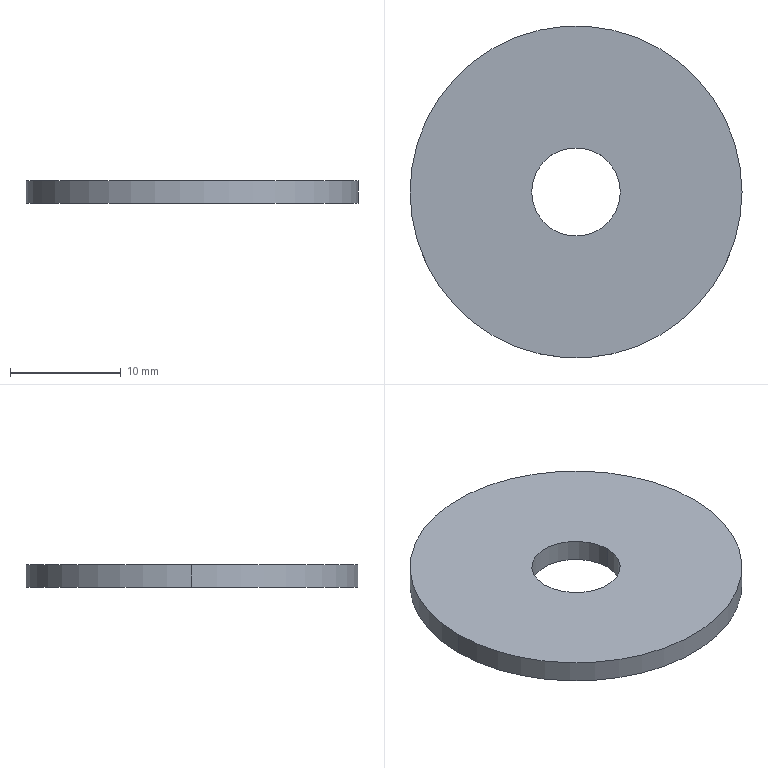Part | STEP file | BCC3 H16_6 | 1 solid | 6 faces | box 30 x 30 x 2 mm | volume 1313 mm3 | cylinder 4 | plane 2 | commonest cylinder face diameters 8 x2 30 x2
STEP:
#1=CARTESIAN_POINT('',(0.,0.,0.));
#2=DIRECTION('',(0.,0.,1.));
#3=DIRECTION('',(1.,0.,0.));
#4=AXIS2_PLACEMENT_3D('',#1,#2,#3);
#5=CARTESIAN_POINT('',(-4.,0.,2.));
#6=VERTEX_POINT('',#5);
#7=CARTESIAN_POINT('',(-4.,0.,0.));
#8=VERTEX_POINT('',#7);
#9=CARTESIAN_POINT('',(-4.,0.,2.));
#10=DIRECTION('',(0.,0.,-1.));
#11=VECTOR('',#10,1.);
#12=LINE('',#9,#11);
#13=CARTESIAN_POINT('',(0.,0.,2.));
#14=DIRECTION('',(0.,0.,-1.));
#15=DIRECTION('',(-1.,0.,0.));
#16=AXIS2_PLACEMENT_3D('',#13,#14,#15);
#17=CYLINDRICAL_SURFACE('',#16,4.);
#18=CARTESIAN_POINT('',(6.283,0.));
#19=DIRECTION('',(0.,1.));
#20=VECTOR('',#19,1.);
#21=LINE('',#18,#20);
#22=(GEOMETRIC_REPRESENTATION_CONTEXT(2)PARAMETRIC_REPRESENTATION_CONTEXT()REPRESENTATION_CONTEXT('',''));
#23=DEFINITIONAL_REPRESENTATION('',(#21),#22);
#24=PCURVE('',#17,#23);
#25=CARTESIAN_POINT('',(0.,0.,2.));
#26=DIRECTION('',(0.,0.,-1.));
#27=DIRECTION('',(-1.,0.,0.));
#28=AXIS2_PLACEMENT_3D('',#25,#26,#27);
#29=CYLINDRICAL_SURFACE('',#28,4.);
#30=CARTESIAN_POINT('',(0.,0.));
#31=DIRECTION('',(0.,1.));
#32=VECTOR('',#31,1.);
#33=LINE('',#30,#32);
#34=(GEOMETRIC_REPRESENTATION_CONTEXT(2)PARAMETRIC_REPRESENTATION_CONTEXT()REPRESENTATION_CONTEXT('',''));
#35=DEFINITIONAL_REPRESENTATION('',(#33),#34);
#36=PCURVE('',#29,#35);
#37=SURFACE_CURVE('',#12,(#24,#36),.PCURVE_S1.);
#38=EDGE_CURVE('',#6,#8,#37,.T.);
#39=ORIENTED_EDGE('',*,*,#38,.T.);
#40=CARTESIAN_POINT('',(4.,0.,0.));
#41=VERTEX_POINT('',#40);
#42=CARTESIAN_POINT('',(0.,0.,0.));
#43=DIRECTION('',(0.,0.,1.));
#44=DIRECTION('',(1.,0.,0.));
#45=AXIS2_PLACEMENT_3D('',#42,#43,#44);
#46=CIRCLE('',#45,4.);
#47=CARTESIAN_POINT('',(9.425,2.));
#48=DIRECTION('',(-1.,0.));
#49=VECTOR('',#48,1.);
#50=LINE('',#47,#49);
#51=(GEOMETRIC_REPRESENTATION_CONTEXT(2)PARAMETRIC_REPRESENTATION_CONTEXT()REPRESENTATION_CONTEXT('',''));
#52=DEFINITIONAL_REPRESENTATION('',(#50),#51);
#53=PCURVE('',#17,#52);
#54=CARTESIAN_POINT('',(0.,0.,0.));
#55=DIRECTION('',(0.,0.,1.));
#56=DIRECTION('',(1.,0.,0.));
#57=AXIS2_PLACEMENT_3D('',#54,#55,#56);
#58=PLANE('',#57);
#59=CARTESIAN_POINT('',(0.,0.));
#60=DIRECTION('',(1.,0.));
#61=AXIS2_PLACEMENT_2D('',#59,#60);
#62=CIRCLE('',#61,4.);
#63=(GEOMETRIC_REPRESENTATION_CONTEXT(2)PARAMETRIC_REPRESENTATION_CONTEXT()REPRESENTATION_CONTEXT('',''));
#64=DEFINITIONAL_REPRESENTATION('',(#62),#63);
#65=PCURVE('',#58,#64);
#66=SURFACE_CURVE('',#46,(#53,#65),.PCURVE_S1.);
#67=EDGE_CURVE('',#8,#41,#66,.T.);
#68=ORIENTED_EDGE('',*,*,#67,.T.);
#69=CARTESIAN_POINT('',(4.,0.,2.));
#70=VERTEX_POINT('',#69);
#71=CARTESIAN_POINT('',(4.,0.,2.));
#72=DIRECTION('',(0.,0.,-1.));
#73=VECTOR('',#72,1.);
#74=LINE('',#71,#73);
#75=CARTESIAN_POINT('',(3.142,0.));
#76=DIRECTION('',(0.,1.));
#77=VECTOR('',#76,1.);
#78=LINE('',#75,#77);
#79=(GEOMETRIC_REPRESENTATION_CONTEXT(2)PARAMETRIC_REPRESENTATION_CONTEXT()REPRESENTATION_CONTEXT('',''));
#80=DEFINITIONAL_REPRESENTATION('',(#78),#79);
#81=PCURVE('',#17,#80);
#82=CARTESIAN_POINT('',(3.142,0.));
#83=DIRECTION('',(0.,1.));
#84=VECTOR('',#83,1.);
#85=LINE('',#82,#84);
#86=(GEOMETRIC_REPRESENTATION_CONTEXT(2)PARAMETRIC_REPRESENTATION_CONTEXT()REPRESENTATION_CONTEXT('',''));
#87=DEFINITIONAL_REPRESENTATION('',(#85),#86);
#88=PCURVE('',#29,#87);
#89=SURFACE_CURVE('',#74,(#81,#88),.PCURVE_S1.);
#90=EDGE_CURVE('',#70,#41,#89,.T.);
#91=ORIENTED_EDGE('',*,*,#90,.F.);
#92=CARTESIAN_POINT('',(0.,0.,2.));
#93=DIRECTION('',(0.,0.,1.));
#94=DIRECTION('',(1.,0.,0.));
#95=AXIS2_PLACEMENT_3D('',#92,#93,#94);
#96=CIRCLE('',#95,4.);
#97=CARTESIAN_POINT('',(9.425,0.));
#98=DIRECTION('',(-1.,0.));
#99=VECTOR('',#98,1.);
#100=LINE('',#97,#99);
#101=(GEOMETRIC_REPRESENTATION_CONTEXT(2)PARAMETRIC_REPRESENTATION_CONTEXT()REPRESENTATION_CONTEXT('',''));
#102=DEFINITIONAL_REPRESENTATION('',(#100),#101);
#103=PCURVE('',#17,#102);
#104=CARTESIAN_POINT('',(0.,0.,2.));
#105=DIRECTION('',(0.,0.,1.));
#106=DIRECTION('',(1.,0.,0.));
#107=AXIS2_PLACEMENT_3D('',#104,#105,#106);
#108=PLANE('',#107);
#109=CARTESIAN_POINT('',(0.,0.));
#110=DIRECTION('',(1.,0.));
#111=AXIS2_PLACEMENT_2D('',#109,#110);
#112=CIRCLE('',#111,4.);
#113=(GEOMETRIC_REPRESENTATION_CONTEXT(2)PARAMETRIC_REPRESENTATION_CONTEXT()REPRESENTATION_CONTEXT('',''));
#114=DEFINITIONAL_REPRESENTATION('',(#112),#113);
#115=PCURVE('',#108,#114);
#116=SURFACE_CURVE('',#96,(#103,#115),.PCURVE_S1.);
#117=EDGE_CURVE('',#6,#70,#116,.T.);
#118=ORIENTED_EDGE('',*,*,#117,.F.);
#119=EDGE_LOOP('',(#39,#68,#91,#118));
#120=FACE_BOUND('',#119,.F.);
#121=ADVANCED_FACE('',(#120),#17,.F.);
#122=CARTESIAN_POINT('',(15.,0.,2.));
#123=VERTEX_POINT('',#122);
#124=CARTESIAN_POINT('',(-15.,0.,2.));
#125=VERTEX_POINT('',#124);
#126=CARTESIAN_POINT('',(0.,0.,2.));
#127=DIRECTION('',(0.,0.,1.));
#128=DIRECTION('',(1.,0.,0.));
#129=AXIS2_PLACEMENT_3D('',#126,#127,#128);
#130=CIRCLE('',#129,15.);
#131=CARTESIAN_POINT('',(0.,0.,2.));
#132=DIRECTION('',(0.,0.,-1.));
#133=DIRECTION('',(-1.,0.,0.));
#134=AXIS2_PLACEMENT_3D('',#131,#132,#133);
#135=CYLINDRICAL_SURFACE('',#134,15.);
#136=CARTESIAN_POINT('',(3.142,0.));
#137=DIRECTION('',(-1.,0.));
#138=VECTOR('',#137,1.);
#139=LINE('',#136,#138);
#140=(GEOMETRIC_REPRESENTATION_CONTEXT(2)PARAMETRIC_REPRESENTATION_CONTEXT()REPRESENTATION_CONTEXT('',''));
#141=DEFINITIONAL_REPRESENTATION('',(#139),#140);
#142=PCURVE('',#135,#141);
#143=CARTESIAN_POINT('',(0.,0.));
#144=DIRECTION('',(1.,0.));
#145=AXIS2_PLACEMENT_2D('',#143,#144);
#146=CIRCLE('',#145,15.);
#147=(GEOMETRIC_REPRESENTATION_CONTEXT(2)PARAMETRIC_REPRESENTATION_CONTEXT()REPRESENTATION_CONTEXT('',''));
#148=DEFINITIONAL_REPRESENTATION('',(#146),#147);
#149=PCURVE('',#108,#148);
#150=SURFACE_CURVE('',#130,(#142,#149),.PCURVE_S1.);
#151=EDGE_CURVE('',#123,#125,#150,.T.);
#152=ORIENTED_EDGE('',*,*,#151,.F.);
#153=CARTESIAN_POINT('',(15.,0.,0.));
#154=VERTEX_POINT('',#153);
#155=CARTESIAN_POINT('',(15.,0.,2.));
#156=DIRECTION('',(0.,0.,-1.));
#157=VECTOR('',#156,1.);
#158=LINE('',#155,#157);
#159=CARTESIAN_POINT('',(3.142,0.));
#160=DIRECTION('',(0.,1.));
#161=VECTOR('',#160,1.);
#162=LINE('',#159,#161);
#163=(GEOMETRIC_REPRESENTATION_CONTEXT(2)PARAMETRIC_REPRESENTATION_CONTEXT()REPRESENTATION_CONTEXT('',''));
#164=DEFINITIONAL_REPRESENTATION('',(#162),#163);
#165=PCURVE('',#135,#164);
#166=CARTESIAN_POINT('',(0.,0.,2.));
#167=DIRECTION('',(0.,0.,-1.));
#168=DIRECTION('',(-1.,0.,0.));
#169=AXIS2_PLACEMENT_3D('',#166,#167,#168);
#170=CYLINDRICAL_SURFACE('',#169,15.);
#171=CARTESIAN_POINT('',(3.142,0.));
#172=DIRECTION('',(0.,1.));
#173=VECTOR('',#172,1.);
#174=LINE('',#171,#173);
#175=(GEOMETRIC_REPRESENTATION_CONTEXT(2)PARAMETRIC_REPRESENTATION_CONTEXT()REPRESENTATION_CONTEXT('',''));
#176=DEFINITIONAL_REPRESENTATION('',(#174),#175);
#177=PCURVE('',#170,#176);
#178=SURFACE_CURVE('',#158,(#165,#177),.PCURVE_S1.);
#179=EDGE_CURVE('',#123,#154,#178,.T.);
#180=ORIENTED_EDGE('',*,*,#179,.T.);
#181=CARTESIAN_POINT('',(-15.,0.,0.));
#182=VERTEX_POINT('',#181);
#183=CARTESIAN_POINT('',(0.,0.,0.));
#184=DIRECTION('',(0.,0.,1.));
#185=DIRECTION('',(1.,0.,0.));
#186=AXIS2_PLACEMENT_3D('',#183,#184,#185);
#187=CIRCLE('',#186,15.);
#188=CARTESIAN_POINT('',(3.142,2.));
#189=DIRECTION('',(-1.,0.));
#190=VECTOR('',#189,1.);
#191=LINE('',#188,#190);
#192=(GEOMETRIC_REPRESENTATION_CONTEXT(2)PARAMETRIC_REPRESENTATION_CONTEXT()REPRESENTATION_CONTEXT('',''));
#193=DEFINITIONAL_REPRESENTATION('',(#191),#192);
#194=PCURVE('',#135,#193);
#195=CARTESIAN_POINT('',(0.,0.));
#196=DIRECTION('',(1.,0.));
#197=AXIS2_PLACEMENT_2D('',#195,#196);
#198=CIRCLE('',#197,15.);
#199=(GEOMETRIC_REPRESENTATION_CONTEXT(2)PARAMETRIC_REPRESENTATION_CONTEXT()REPRESENTATION_CONTEXT('',''));
#200=DEFINITIONAL_REPRESENTATION('',(#198),#199);
#201=PCURVE('',#58,#200);
#202=SURFACE_CURVE('',#187,(#194,#201),.PCURVE_S1.);
#203=EDGE_CURVE('',#154,#182,#202,.T.);
#204=ORIENTED_EDGE('',*,*,#203,.T.);
#205=CARTESIAN_POINT('',(-15.,0.,2.));
#206=DIRECTION('',(0.,0.,-1.));
#207=VECTOR('',#206,1.);
#208=LINE('',#205,#207);
#209=CARTESIAN_POINT('',(0.,0.));
#210=DIRECTION('',(0.,1.));
#211=VECTOR('',#210,1.);
#212=LINE('',#209,#211);
#213=(GEOMETRIC_REPRESENTATION_CONTEXT(2)PARAMETRIC_REPRESENTATION_CONTEXT()REPRESENTATION_CONTEXT('',''));
#214=DEFINITIONAL_REPRESENTATION('',(#212),#213);
#215=PCURVE('',#135,#214);
#216=CARTESIAN_POINT('',(6.283,0.));
#217=DIRECTION('',(0.,1.));
#218=VECTOR('',#217,1.);
#219=LINE('',#216,#218);
#220=(GEOMETRIC_REPRESENTATION_CONTEXT(2)PARAMETRIC_REPRESENTATION_CONTEXT()REPRESENTATION_CONTEXT('',''));
#221=DEFINITIONAL_REPRESENTATION('',(#219),#220);
#222=PCURVE('',#170,#221);
#223=SURFACE_CURVE('',#208,(#215,#222),.PCURVE_S1.);
#224=EDGE_CURVE('',#125,#182,#223,.T.);
#225=ORIENTED_EDGE('',*,*,#224,.F.);
#226=EDGE_LOOP('',(#152,#180,#204,#225));
#227=FACE_BOUND('',#226,.T.);
#228=ADVANCED_FACE('',(#227),#135,.T.);
#229=CARTESIAN_POINT('',(0.,0.,2.));
#230=DIRECTION('',(0.,0.,1.));
#231=DIRECTION('',(1.,0.,0.));
#232=AXIS2_PLACEMENT_3D('',#229,#230,#231);
#233=CIRCLE('',#232,15.);
#234=CARTESIAN_POINT('',(0.,0.));
#235=DIRECTION('',(1.,0.));
#236=AXIS2_PLACEMENT_2D('',#234,#235);
#237=CIRCLE('',#236,15.);
#238=(GEOMETRIC_REPRESENTATION_CONTEXT(2)PARAMETRIC_REPRESENTATION_CONTEXT()REPRESENTATION_CONTEXT('',''));
#239=DEFINITIONAL_REPRESENTATION('',(#237),#238);
#240=PCURVE('',#108,#239);
#241=CARTESIAN_POINT('',(9.425,0.));
#242=DIRECTION('',(-1.,0.));
#243=VECTOR('',#242,1.);
#244=LINE('',#241,#243);
#245=(GEOMETRIC_REPRESENTATION_CONTEXT(2)PARAMETRIC_REPRESENTATION_CONTEXT()REPRESENTATION_CONTEXT('',''));
#246=DEFINITIONAL_REPRESENTATION('',(#244),#245);
#247=PCURVE('',#170,#246);
#248=SURFACE_CURVE('',#233,(#240,#247),.PCURVE_S1.);
#249=EDGE_CURVE('',#125,#123,#248,.T.);
#250=ORIENTED_EDGE('',*,*,#249,.T.);
#251=ORIENTED_EDGE('',*,*,#151,.T.);
#252=EDGE_LOOP('',(#250,#251));
#253=FACE_BOUND('',#252,.T.);
#254=ORIENTED_EDGE('',*,*,#117,.F.);
#255=CARTESIAN_POINT('',(0.,0.,2.));
#256=DIRECTION('',(0.,0.,1.));
#257=DIRECTION('',(1.,0.,0.));
#258=AXIS2_PLACEMENT_3D('',#255,#256,#257);
#259=CIRCLE('',#258,4.);
#260=CARTESIAN_POINT('',(0.,0.));
#261=DIRECTION('',(1.,0.));
#262=AXIS2_PLACEMENT_2D('',#260,#261);
#263=CIRCLE('',#262,4.);
#264=(GEOMETRIC_REPRESENTATION_CONTEXT(2)PARAMETRIC_REPRESENTATION_CONTEXT()REPRESENTATION_CONTEXT('',''));
#265=DEFINITIONAL_REPRESENTATION('',(#263),#264);
#266=PCURVE('',#108,#265);
#267=CARTESIAN_POINT('',(3.142,0.));
#268=DIRECTION('',(-1.,0.));
#269=VECTOR('',#268,1.);
#270=LINE('',#267,#269);
#271=(GEOMETRIC_REPRESENTATION_CONTEXT(2)PARAMETRIC_REPRESENTATION_CONTEXT()REPRESENTATION_CONTEXT('',''));
#272=DEFINITIONAL_REPRESENTATION('',(#270),#271);
#273=PCURVE('',#29,#272);
#274=SURFACE_CURVE('',#259,(#266,#273),.PCURVE_S1.);
#275=EDGE_CURVE('',#70,#6,#274,.T.);
#276=ORIENTED_EDGE('',*,*,#275,.F.);
#277=EDGE_LOOP('',(#254,#276));
#278=FACE_BOUND('',#277,.T.);
#279=ADVANCED_FACE('',(#253,#278),#108,.T.);
#280=CARTESIAN_POINT('',(0.,0.,0.));
#281=DIRECTION('',(0.,0.,1.));
#282=DIRECTION('',(1.,0.,0.));
#283=AXIS2_PLACEMENT_3D('',#280,#281,#282);
#284=CIRCLE('',#283,15.);
#285=CARTESIAN_POINT('',(0.,0.));
#286=DIRECTION('',(1.,0.));
#287=AXIS2_PLACEMENT_2D('',#285,#286);
#288=CIRCLE('',#287,15.);
#289=(GEOMETRIC_REPRESENTATION_CONTEXT(2)PARAMETRIC_REPRESENTATION_CONTEXT()REPRESENTATION_CONTEXT('',''));
#290=DEFINITIONAL_REPRESENTATION('',(#288),#289);
#291=PCURVE('',#58,#290);
#292=CARTESIAN_POINT('',(9.425,2.));
#293=DIRECTION('',(-1.,0.));
#294=VECTOR('',#293,1.);
#295=LINE('',#292,#294);
#296=(GEOMETRIC_REPRESENTATION_CONTEXT(2)PARAMETRIC_REPRESENTATION_CONTEXT()REPRESENTATION_CONTEXT('',''));
#297=DEFINITIONAL_REPRESENTATION('',(#295),#296);
#298=PCURVE('',#170,#297);
#299=SURFACE_CURVE('',#284,(#291,#298),.PCURVE_S1.);
#300=EDGE_CURVE('',#182,#154,#299,.T.);
#301=ORIENTED_EDGE('',*,*,#300,.F.);
#302=ORIENTED_EDGE('',*,*,#203,.F.);
#303=EDGE_LOOP('',(#301,#302));
#304=FACE_BOUND('',#303,.T.);
#305=ORIENTED_EDGE('',*,*,#67,.T.);
#306=CARTESIAN_POINT('',(0.,0.,0.));
#307=DIRECTION('',(0.,0.,1.));
#308=DIRECTION('',(1.,0.,0.));
#309=AXIS2_PLACEMENT_3D('',#306,#307,#308);
#310=CIRCLE('',#309,4.);
#311=CARTESIAN_POINT('',(0.,0.));
#312=DIRECTION('',(1.,0.));
#313=AXIS2_PLACEMENT_2D('',#311,#312);
#314=CIRCLE('',#313,4.);
#315=(GEOMETRIC_REPRESENTATION_CONTEXT(2)PARAMETRIC_REPRESENTATION_CONTEXT()REPRESENTATION_CONTEXT('',''));
#316=DEFINITIONAL_REPRESENTATION('',(#314),#315);
#317=PCURVE('',#58,#316);
#318=CARTESIAN_POINT('',(3.142,2.));
#319=DIRECTION('',(-1.,0.));
#320=VECTOR('',#319,1.);
#321=LINE('',#318,#320);
#322=(GEOMETRIC_REPRESENTATION_CONTEXT(2)PARAMETRIC_REPRESENTATION_CONTEXT()REPRESENTATION_CONTEXT('',''));
#323=DEFINITIONAL_REPRESENTATION('',(#321),#322);
#324=PCURVE('',#29,#323);
#325=SURFACE_CURVE('',#310,(#317,#324),.PCURVE_S1.);
#326=EDGE_CURVE('',#41,#8,#325,.T.);
#327=ORIENTED_EDGE('',*,*,#326,.T.);
#328=EDGE_LOOP('',(#305,#327));
#329=FACE_BOUND('',#328,.T.);
#330=ADVANCED_FACE('',(#304,#329),#58,.F.);
#331=ORIENTED_EDGE('',*,*,#179,.F.);
#332=ORIENTED_EDGE('',*,*,#249,.F.);
#333=ORIENTED_EDGE('',*,*,#224,.T.);
#334=ORIENTED_EDGE('',*,*,#300,.T.);
#335=EDGE_LOOP('',(#331,#332,#333,#334));
#336=FACE_BOUND('',#335,.T.);
#337=ADVANCED_FACE('',(#336),#170,.T.);
#338=ORIENTED_EDGE('',*,*,#326,.T.);
#339=ORIENTED_EDGE('',*,*,#38,.F.);
#340=ORIENTED_EDGE('',*,*,#275,.F.);
#341=ORIENTED_EDGE('',*,*,#90,.T.);
#342=EDGE_LOOP('',(#338,#339,#340,#341));
#343=FACE_BOUND('',#342,.F.);
#344=ADVANCED_FACE('',(#343),#29,.F.);
#345=CLOSED_SHELL('',(#121,#228,#279,#330,#337,#344));
#346=MANIFOLD_SOLID_BREP('',#345);
#347=(LENGTH_UNIT()NAMED_UNIT(*)SI_UNIT(.MILLI.,.METRE.));
#348=UNCERTAINTY_MEASURE_WITH_UNIT(LENGTH_MEASURE(0.0000001),#347,'','');
#349=(NAMED_UNIT(*)PLANE_ANGLE_UNIT()SI_UNIT($,.RADIAN.));
#350=(NAMED_UNIT(*)SI_UNIT($,.STERADIAN.)SOLID_ANGLE_UNIT());
#351=(GEOMETRIC_REPRESENTATION_CONTEXT(3)GLOBAL_UNCERTAINTY_ASSIGNED_CONTEXT((#348))GLOBAL_UNIT_ASSIGNED_CONTEXT((#347,#349,#350))REPRESENTATION_CONTEXT('',''));
#352=ADVANCED_BREP_SHAPE_REPRESENTATION('',(#4,#346),#351);